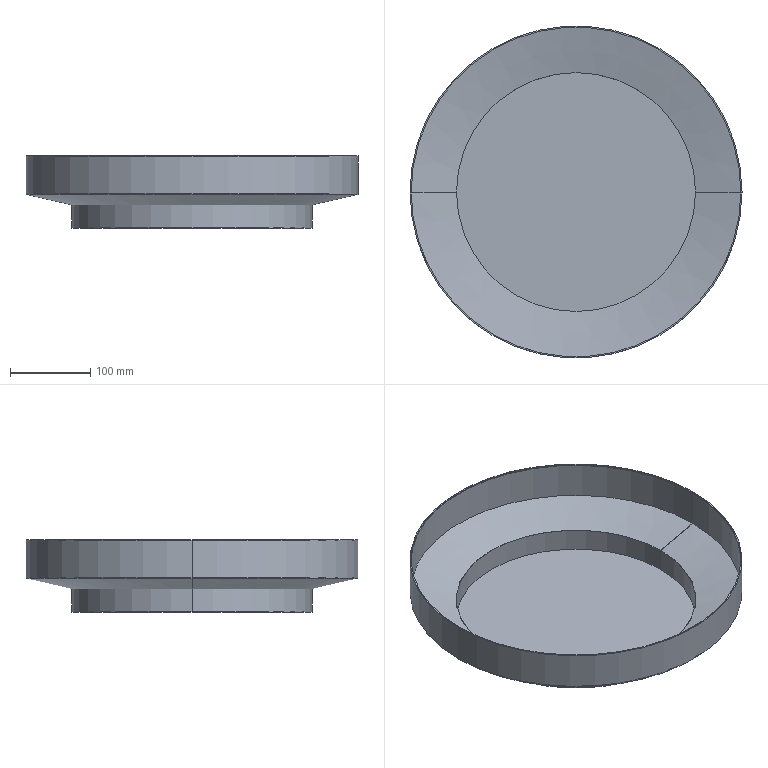Part | NX | 1 solid | 18 faces | box 414 x 414 x 90 mm | volume 225156 mm3 | cylinder 10 | plane 4 | cone 4 | commonest cylinder face diameters 298 x2 300 x2 411 x2 412 x2 414 x2
STEP:
#1=CARTESIAN_POINT('',(-186.483,-361.015,34.752));
#2=VERTEX_POINT('',#1);
#3=CARTESIAN_POINT('',(113.517,-361.015,34.752));
#4=VERTEX_POINT('',#3);
#5=CARTESIAN_POINT('',(-36.483,-361.015,34.752));
#6=DIRECTION('',(0.,0.,-1.));
#7=DIRECTION('',(1.,0.,0.));
#8=AXIS2_PLACEMENT_3D('',#5,#6,#7);
#9=CIRCLE('',#8,150.);
#10=EDGE_CURVE('',#2,#4,#9,.T.);
#11=ORIENTED_EDGE('',*,*,#10,.T.);
#12=CARTESIAN_POINT('',(-36.483,-361.015,34.752));
#13=DIRECTION('',(0.,0.,-1.));
#14=DIRECTION('',(1.,0.,0.));
#15=AXIS2_PLACEMENT_3D('',#12,#13,#14);
#16=CIRCLE('',#15,150.);
#17=EDGE_CURVE('',#4,#2,#16,.T.);
#18=ORIENTED_EDGE('',*,*,#17,.T.);
#19=EDGE_LOOP('',(#11,#18));
#20=FACE_BOUND('',#19,.T.);
#21=CARTESIAN_POINT('',(38.517,-361.015,34.752));
#22=DIRECTION('',(0.,0.,-1.));
#23=DIRECTION('',(0.,-1.,0.));
#24=AXIS2_PLACEMENT_3D('',#21,#22,#23);
#25=PLANE('',#24);
#26=ADVANCED_FACE('',(#20),#25,.T.);
#27=CARTESIAN_POINT('',(-186.483,-361.015,63.752));
#28=VERTEX_POINT('',#27);
#29=CARTESIAN_POINT('',(113.517,-361.015,63.752));
#30=VERTEX_POINT('',#29);
#31=CARTESIAN_POINT('',(-36.483,-361.015,63.752));
#32=DIRECTION('',(0.,0.,-1.));
#33=DIRECTION('',(1.,0.,0.));
#34=AXIS2_PLACEMENT_3D('',#31,#32,#33);
#35=CIRCLE('',#34,150.);
#36=EDGE_CURVE('',#28,#30,#35,.T.);
#37=ORIENTED_EDGE('',*,*,#36,.T.);
#38=CARTESIAN_POINT('',(113.517,-361.015,49.252));
#39=DIRECTION('',(0.,0.,1.));
#40=VECTOR('',#39,1000.);
#41=LINE('',#38,#40);
#42=EDGE_CURVE('',#4,#30,#41,.T.);
#43=ORIENTED_EDGE('',*,*,#42,.F.);
#44=ORIENTED_EDGE('',*,*,#10,.F.);
#45=CARTESIAN_POINT('',(-186.483,-361.015,49.252));
#46=DIRECTION('',(0.,0.,1.));
#47=VECTOR('',#46,1000.);
#48=LINE('',#45,#47);
#49=EDGE_CURVE('',#2,#28,#48,.T.);
#50=ORIENTED_EDGE('',*,*,#49,.T.);
#51=EDGE_LOOP('',(#37,#43,#44,#50));
#52=FACE_BOUND('',#51,.T.);
#53=CARTESIAN_POINT('',(-36.483,-361.015,49.252));
#54=DIRECTION('',(0.,0.,1.));
#55=DIRECTION('',(1.,0.,0.));
#56=AXIS2_PLACEMENT_3D('',#53,#54,#55);
#57=CYLINDRICAL_SURFACE('',#56,150.);
#58=ADVANCED_FACE('',(#52),#57,.T.);
#59=CARTESIAN_POINT('',(-243.483,-361.015,76.752));
#60=VERTEX_POINT('',#59);
#61=CARTESIAN_POINT('',(170.517,-361.015,76.752));
#62=VERTEX_POINT('',#61);
#63=CARTESIAN_POINT('',(-36.483,-361.015,76.752));
#64=DIRECTION('',(0.,0.,-1.));
#65=DIRECTION('',(1.,0.,0.));
#66=AXIS2_PLACEMENT_3D('',#63,#64,#65);
#67=CIRCLE('',#66,207.);
#68=EDGE_CURVE('',#60,#62,#67,.T.);
#69=ORIENTED_EDGE('',*,*,#68,.T.);
#70=CARTESIAN_POINT('',(170.517,-361.015,76.752));
#71=DIRECTION('',(0.975,0.,0.2224));
#72=VECTOR('',#71,1000.);
#73=LINE('',#70,#72);
#74=EDGE_CURVE('',#30,#62,#73,.T.);
#75=ORIENTED_EDGE('',*,*,#74,.F.);
#76=ORIENTED_EDGE('',*,*,#36,.F.);
#77=CARTESIAN_POINT('',(-243.483,-361.015,76.752));
#78=DIRECTION('',(-0.975,0.,0.2224));
#79=VECTOR('',#78,1000.);
#80=LINE('',#77,#79);
#81=EDGE_CURVE('',#28,#60,#80,.T.);
#82=ORIENTED_EDGE('',*,*,#81,.T.);
#83=EDGE_LOOP('',(#69,#75,#76,#82));
#84=FACE_BOUND('',#83,.T.);
#85=CARTESIAN_POINT('',(-36.483,-361.015,76.752));
#86=DIRECTION('',(0.,0.,1.));
#87=DIRECTION('',(1.,0.,0.));
#88=AXIS2_PLACEMENT_3D('',#85,#86,#87);
#89=CONICAL_SURFACE('',#88,207.,1.347);
#90=ADVANCED_FACE('',(#84),#89,.T.);
#91=CARTESIAN_POINT('',(-243.483,-361.015,124.752));
#92=VERTEX_POINT('',#91);
#93=CARTESIAN_POINT('',(170.517,-361.015,124.752));
#94=VERTEX_POINT('',#93);
#95=CARTESIAN_POINT('',(-36.483,-361.015,124.752));
#96=DIRECTION('',(0.,0.,-1.));
#97=DIRECTION('',(1.,0.,0.));
#98=AXIS2_PLACEMENT_3D('',#95,#96,#97);
#99=CIRCLE('',#98,207.);
#100=EDGE_CURVE('',#92,#94,#99,.T.);
#101=ORIENTED_EDGE('',*,*,#100,.T.);
#102=CARTESIAN_POINT('',(170.517,-361.015,100.752));
#103=DIRECTION('',(0.,0.,1.));
#104=VECTOR('',#103,1000.);
#105=LINE('',#102,#104);
#106=EDGE_CURVE('',#62,#94,#105,.T.);
#107=ORIENTED_EDGE('',*,*,#106,.F.);
#108=ORIENTED_EDGE('',*,*,#68,.F.);
#109=CARTESIAN_POINT('',(-243.483,-361.015,100.752));
#110=DIRECTION('',(0.,0.,1.));
#111=VECTOR('',#110,1000.);
#112=LINE('',#109,#111);
#113=EDGE_CURVE('',#60,#92,#112,.T.);
#114=ORIENTED_EDGE('',*,*,#113,.T.);
#115=EDGE_LOOP('',(#101,#107,#108,#114));
#116=FACE_BOUND('',#115,.T.);
#117=CARTESIAN_POINT('',(-36.483,-361.015,100.752));
#118=DIRECTION('',(0.,0.,1.));
#119=DIRECTION('',(1.,0.,0.));
#120=AXIS2_PLACEMENT_3D('',#117,#118,#119);
#121=CYLINDRICAL_SURFACE('',#120,207.);
#122=ADVANCED_FACE('',(#116),#121,.T.);
#123=ORIENTED_EDGE('',*,*,#100,.F.);
#124=CARTESIAN_POINT('',(-36.483,-361.015,124.752));
#125=DIRECTION('',(0.,0.,-1.));
#126=DIRECTION('',(1.,0.,0.));
#127=AXIS2_PLACEMENT_3D('',#124,#125,#126);
#128=CIRCLE('',#127,207.);
#129=EDGE_CURVE('',#94,#92,#128,.T.);
#130=ORIENTED_EDGE('',*,*,#129,.F.);
#131=EDGE_LOOP('',(#123,#130));
#132=FACE_BOUND('',#131,.T.);
#133=CARTESIAN_POINT('',(-241.983,-361.015,124.752));
#134=VERTEX_POINT('',#133);
#135=CARTESIAN_POINT('',(169.017,-361.015,124.752));
#136=VERTEX_POINT('',#135);
#137=CARTESIAN_POINT('',(-36.483,-361.015,124.752));
#138=DIRECTION('',(0.,0.,1.));
#139=DIRECTION('',(1.,0.,0.));
#140=AXIS2_PLACEMENT_3D('',#137,#138,#139);
#141=CIRCLE('',#140,205.5);
#142=EDGE_CURVE('',#134,#136,#141,.T.);
#143=ORIENTED_EDGE('',*,*,#142,.F.);
#144=CARTESIAN_POINT('',(-36.483,-361.015,124.752));
#145=DIRECTION('',(0.,0.,1.));
#146=DIRECTION('',(1.,0.,0.));
#147=AXIS2_PLACEMENT_3D('',#144,#145,#146);
#148=CIRCLE('',#147,205.5);
#149=EDGE_CURVE('',#136,#134,#148,.T.);
#150=ORIENTED_EDGE('',*,*,#149,.F.);
#151=EDGE_LOOP('',(#143,#150));
#152=FACE_BOUND('',#151,.T.);
#153=CARTESIAN_POINT('',(67.017,-361.015,124.752));
#154=DIRECTION('',(0.,0.,1.));
#155=DIRECTION('',(1.,0.,0.));
#156=AXIS2_PLACEMENT_3D('',#153,#154,#155);
#157=PLANE('',#156);
#158=ADVANCED_FACE('',(#132,#152),#157,.T.);
#159=CARTESIAN_POINT('',(-241.983,-361.015,123.752));
#160=VERTEX_POINT('',#159);
#161=CARTESIAN_POINT('',(169.017,-361.015,123.752));
#162=VERTEX_POINT('',#161);
#163=CARTESIAN_POINT('',(-36.483,-361.015,123.752));
#164=DIRECTION('',(0.,0.,1.));
#165=DIRECTION('',(1.,0.,0.));
#166=AXIS2_PLACEMENT_3D('',#163,#164,#165);
#167=CIRCLE('',#166,205.5);
#168=EDGE_CURVE('',#160,#162,#167,.T.);
#169=ORIENTED_EDGE('',*,*,#168,.F.);
#170=CARTESIAN_POINT('',(-241.983,-361.015,100.752));
#171=DIRECTION('',(0.,0.,1.));
#172=VECTOR('',#171,1000.);
#173=LINE('',#170,#172);
#174=EDGE_CURVE('',#160,#134,#173,.T.);
#175=ORIENTED_EDGE('',*,*,#174,.T.);
#176=ORIENTED_EDGE('',*,*,#142,.T.);
#177=CARTESIAN_POINT('',(169.017,-361.015,100.752));
#178=DIRECTION('',(0.,0.,1.));
#179=VECTOR('',#178,1000.);
#180=LINE('',#177,#179);
#181=EDGE_CURVE('',#162,#136,#180,.T.);
#182=ORIENTED_EDGE('',*,*,#181,.F.);
#183=EDGE_LOOP('',(#169,#175,#176,#182));
#184=FACE_BOUND('',#183,.T.);
#185=CARTESIAN_POINT('',(-36.483,-361.015,100.752));
#186=DIRECTION('',(0.,0.,1.));
#187=DIRECTION('',(1.,0.,0.));
#188=AXIS2_PLACEMENT_3D('',#185,#186,#187);
#189=CYLINDRICAL_SURFACE('',#188,205.5);
#190=ADVANCED_FACE('',(#184),#189,.F.);
#191=CARTESIAN_POINT('',(-242.483,-361.015,123.752));
#192=VERTEX_POINT('',#191);
#193=CARTESIAN_POINT('',(169.517,-361.015,123.752));
#194=VERTEX_POINT('',#193);
#195=CARTESIAN_POINT('',(-36.483,-361.015,123.752));
#196=DIRECTION('',(0.,0.,1.));
#197=DIRECTION('',(1.,0.,0.));
#198=AXIS2_PLACEMENT_3D('',#195,#196,#197);
#199=CIRCLE('',#198,206.);
#200=EDGE_CURVE('',#192,#194,#199,.T.);
#201=ORIENTED_EDGE('',*,*,#200,.F.);
#202=CARTESIAN_POINT('',(-36.483,-361.015,123.752));
#203=DIRECTION('',(0.,0.,1.));
#204=DIRECTION('',(1.,0.,0.));
#205=AXIS2_PLACEMENT_3D('',#202,#203,#204);
#206=CIRCLE('',#205,206.);
#207=EDGE_CURVE('',#194,#192,#206,.T.);
#208=ORIENTED_EDGE('',*,*,#207,.F.);
#209=EDGE_LOOP('',(#201,#208));
#210=FACE_BOUND('',#209,.T.);
#211=ORIENTED_EDGE('',*,*,#168,.T.);
#212=CARTESIAN_POINT('',(-36.483,-361.015,123.752));
#213=DIRECTION('',(0.,0.,1.));
#214=DIRECTION('',(1.,0.,0.));
#215=AXIS2_PLACEMENT_3D('',#212,#213,#214);
#216=CIRCLE('',#215,205.5);
#217=EDGE_CURVE('',#162,#160,#216,.T.);
#218=ORIENTED_EDGE('',*,*,#217,.T.);
#219=EDGE_LOOP('',(#211,#218));
#220=FACE_BOUND('',#219,.T.);
#221=CARTESIAN_POINT('',(67.017,-361.015,123.752));
#222=DIRECTION('',(0.,0.,1.));
#223=DIRECTION('',(1.,0.,0.));
#224=AXIS2_PLACEMENT_3D('',#221,#222,#223);
#225=PLANE('',#224);
#226=ADVANCED_FACE('',(#210,#220),#225,.F.);
#227=ORIENTED_EDGE('',*,*,#200,.T.);
#228=CARTESIAN_POINT('',(169.517,-361.015,77.549));
#229=VERTEX_POINT('',#228);
#230=CARTESIAN_POINT('',(169.517,-361.015,100.752));
#231=DIRECTION('',(0.,0.,1.));
#232=VECTOR('',#231,1000.);
#233=LINE('',#230,#232);
#234=EDGE_CURVE('',#229,#194,#233,.T.);
#235=ORIENTED_EDGE('',*,*,#234,.F.);
#236=CARTESIAN_POINT('',(-242.483,-361.015,77.549));
#237=VERTEX_POINT('',#236);
#238=CARTESIAN_POINT('',(-36.483,-361.015,77.549));
#239=DIRECTION('',(0.,0.,1.));
#240=DIRECTION('',(1.,0.,0.));
#241=AXIS2_PLACEMENT_3D('',#238,#239,#240);
#242=CIRCLE('',#241,206.);
#243=EDGE_CURVE('',#237,#229,#242,.T.);
#244=ORIENTED_EDGE('',*,*,#243,.F.);
#245=CARTESIAN_POINT('',(-242.483,-361.015,100.752));
#246=DIRECTION('',(0.,0.,1.));
#247=VECTOR('',#246,1000.);
#248=LINE('',#245,#247);
#249=EDGE_CURVE('',#237,#192,#248,.T.);
#250=ORIENTED_EDGE('',*,*,#249,.T.);
#251=EDGE_LOOP('',(#227,#235,#244,#250));
#252=FACE_BOUND('',#251,.T.);
#253=CARTESIAN_POINT('',(-36.483,-361.015,100.752));
#254=DIRECTION('',(0.,0.,1.));
#255=DIRECTION('',(1.,0.,0.));
#256=AXIS2_PLACEMENT_3D('',#253,#254,#255);
#257=CYLINDRICAL_SURFACE('',#256,206.);
#258=ADVANCED_FACE('',(#252),#257,.F.);
#259=ORIENTED_EDGE('',*,*,#243,.T.);
#260=CARTESIAN_POINT('',(112.517,-361.015,64.549));
#261=VERTEX_POINT('',#260);
#262=CARTESIAN_POINT('',(170.517,-361.015,77.777));
#263=DIRECTION('',(0.975,0.,0.2224));
#264=VECTOR('',#263,1000.);
#265=LINE('',#262,#264);
#266=EDGE_CURVE('',#261,#229,#265,.T.);
#267=ORIENTED_EDGE('',*,*,#266,.F.);
#268=CARTESIAN_POINT('',(-185.483,-361.015,64.549));
#269=VERTEX_POINT('',#268);
#270=CARTESIAN_POINT('',(-36.483,-361.015,64.549));
#271=DIRECTION('',(0.,0.,1.));
#272=DIRECTION('',(1.,0.,0.));
#273=AXIS2_PLACEMENT_3D('',#270,#271,#272);
#274=CIRCLE('',#273,149.);
#275=EDGE_CURVE('',#269,#261,#274,.T.);
#276=ORIENTED_EDGE('',*,*,#275,.F.);
#277=CARTESIAN_POINT('',(-243.483,-361.015,77.777));
#278=DIRECTION('',(-0.975,0.,0.2224));
#279=VECTOR('',#278,1000.);
#280=LINE('',#277,#279);
#281=EDGE_CURVE('',#269,#237,#280,.T.);
#282=ORIENTED_EDGE('',*,*,#281,.T.);
#283=EDGE_LOOP('',(#259,#267,#276,#282));
#284=FACE_BOUND('',#283,.T.);
#285=CARTESIAN_POINT('',(-36.483,-361.015,77.777));
#286=DIRECTION('',(0.,0.,1.));
#287=DIRECTION('',(1.,0.,0.));
#288=AXIS2_PLACEMENT_3D('',#285,#286,#287);
#289=CONICAL_SURFACE('',#288,207.,1.347);
#290=ADVANCED_FACE('',(#284),#289,.F.);
#291=ORIENTED_EDGE('',*,*,#275,.T.);
#292=CARTESIAN_POINT('',(112.517,-361.015,35.752));
#293=VERTEX_POINT('',#292);
#294=CARTESIAN_POINT('',(112.517,-361.015,49.252));
#295=DIRECTION('',(0.,0.,1.));
#296=VECTOR('',#295,1000.);
#297=LINE('',#294,#296);
#298=EDGE_CURVE('',#293,#261,#297,.T.);
#299=ORIENTED_EDGE('',*,*,#298,.F.);
#300=CARTESIAN_POINT('',(-185.483,-361.015,35.752));
#301=VERTEX_POINT('',#300);
#302=CARTESIAN_POINT('',(-36.483,-361.015,35.752));
#303=DIRECTION('',(0.,0.,1.));
#304=DIRECTION('',(1.,0.,0.));
#305=AXIS2_PLACEMENT_3D('',#302,#303,#304);
#306=CIRCLE('',#305,149.);
#307=EDGE_CURVE('',#301,#293,#306,.T.);
#308=ORIENTED_EDGE('',*,*,#307,.F.);
#309=CARTESIAN_POINT('',(-185.483,-361.015,49.252));
#310=DIRECTION('',(0.,0.,1.));
#311=VECTOR('',#310,1000.);
#312=LINE('',#309,#311);
#313=EDGE_CURVE('',#301,#269,#312,.T.);
#314=ORIENTED_EDGE('',*,*,#313,.T.);
#315=EDGE_LOOP('',(#291,#299,#308,#314));
#316=FACE_BOUND('',#315,.T.);
#317=CARTESIAN_POINT('',(-36.483,-361.015,49.252));
#318=DIRECTION('',(0.,0.,1.));
#319=DIRECTION('',(1.,0.,0.));
#320=AXIS2_PLACEMENT_3D('',#317,#318,#319);
#321=CYLINDRICAL_SURFACE('',#320,149.);
#322=ADVANCED_FACE('',(#316),#321,.F.);
#323=ORIENTED_EDGE('',*,*,#307,.T.);
#324=CARTESIAN_POINT('',(-36.483,-361.015,35.752));
#325=DIRECTION('',(0.,0.,1.));
#326=DIRECTION('',(1.,0.,0.));
#327=AXIS2_PLACEMENT_3D('',#324,#325,#326);
#328=CIRCLE('',#327,149.);
#329=EDGE_CURVE('',#293,#301,#328,.T.);
#330=ORIENTED_EDGE('',*,*,#329,.T.);
#331=EDGE_LOOP('',(#323,#330));
#332=FACE_BOUND('',#331,.T.);
#333=CARTESIAN_POINT('',(38.517,-361.015,35.752));
#334=DIRECTION('',(0.,0.,-1.));
#335=DIRECTION('',(0.,-1.,0.));
#336=AXIS2_PLACEMENT_3D('',#333,#334,#335);
#337=PLANE('',#336);
#338=ADVANCED_FACE('',(#332),#337,.F.);
#339=ORIENTED_EDGE('',*,*,#234,.T.);
#340=ORIENTED_EDGE('',*,*,#207,.T.);
#341=ORIENTED_EDGE('',*,*,#249,.F.);
#342=CARTESIAN_POINT('',(-36.483,-361.015,77.549));
#343=DIRECTION('',(0.,0.,1.));
#344=DIRECTION('',(1.,0.,0.));
#345=AXIS2_PLACEMENT_3D('',#342,#343,#344);
#346=CIRCLE('',#345,206.);
#347=EDGE_CURVE('',#229,#237,#346,.T.);
#348=ORIENTED_EDGE('',*,*,#347,.F.);
#349=EDGE_LOOP('',(#339,#340,#341,#348));
#350=FACE_BOUND('',#349,.T.);
#351=CARTESIAN_POINT('',(-36.483,-361.015,100.752));
#352=DIRECTION('',(0.,0.,1.));
#353=DIRECTION('',(1.,0.,0.));
#354=AXIS2_PLACEMENT_3D('',#351,#352,#353);
#355=CYLINDRICAL_SURFACE('',#354,206.);
#356=ADVANCED_FACE('',(#350),#355,.F.);
#357=ORIENTED_EDGE('',*,*,#181,.T.);
#358=ORIENTED_EDGE('',*,*,#149,.T.);
#359=ORIENTED_EDGE('',*,*,#174,.F.);
#360=ORIENTED_EDGE('',*,*,#217,.F.);
#361=EDGE_LOOP('',(#357,#358,#359,#360));
#362=FACE_BOUND('',#361,.T.);
#363=CARTESIAN_POINT('',(-36.483,-361.015,100.752));
#364=DIRECTION('',(0.,0.,1.));
#365=DIRECTION('',(1.,0.,0.));
#366=AXIS2_PLACEMENT_3D('',#363,#364,#365);
#367=CYLINDRICAL_SURFACE('',#366,205.5);
#368=ADVANCED_FACE('',(#362),#367,.F.);
#369=ORIENTED_EDGE('',*,*,#106,.T.);
#370=ORIENTED_EDGE('',*,*,#129,.T.);
#371=ORIENTED_EDGE('',*,*,#113,.F.);
#372=CARTESIAN_POINT('',(-36.483,-361.015,76.752));
#373=DIRECTION('',(0.,0.,-1.));
#374=DIRECTION('',(1.,0.,0.));
#375=AXIS2_PLACEMENT_3D('',#372,#373,#374);
#376=CIRCLE('',#375,207.);
#377=EDGE_CURVE('',#62,#60,#376,.T.);
#378=ORIENTED_EDGE('',*,*,#377,.F.);
#379=EDGE_LOOP('',(#369,#370,#371,#378));
#380=FACE_BOUND('',#379,.T.);
#381=CARTESIAN_POINT('',(-36.483,-361.015,100.752));
#382=DIRECTION('',(0.,0.,1.));
#383=DIRECTION('',(1.,0.,0.));
#384=AXIS2_PLACEMENT_3D('',#381,#382,#383);
#385=CYLINDRICAL_SURFACE('',#384,207.);
#386=ADVANCED_FACE('',(#380),#385,.T.);
#387=ORIENTED_EDGE('',*,*,#298,.T.);
#388=CARTESIAN_POINT('',(-36.483,-361.015,64.549));
#389=DIRECTION('',(0.,0.,1.));
#390=DIRECTION('',(1.,0.,0.));
#391=AXIS2_PLACEMENT_3D('',#388,#389,#390);
#392=CIRCLE('',#391,149.);
#393=EDGE_CURVE('',#261,#269,#392,.T.);
#394=ORIENTED_EDGE('',*,*,#393,.T.);
#395=ORIENTED_EDGE('',*,*,#313,.F.);
#396=ORIENTED_EDGE('',*,*,#329,.F.);
#397=EDGE_LOOP('',(#387,#394,#395,#396));
#398=FACE_BOUND('',#397,.T.);
#399=CARTESIAN_POINT('',(-36.483,-361.015,49.252));
#400=DIRECTION('',(0.,0.,1.));
#401=DIRECTION('',(1.,0.,0.));
#402=AXIS2_PLACEMENT_3D('',#399,#400,#401);
#403=CYLINDRICAL_SURFACE('',#402,149.);
#404=ADVANCED_FACE('',(#398),#403,.F.);
#405=ORIENTED_EDGE('',*,*,#74,.T.);
#406=ORIENTED_EDGE('',*,*,#377,.T.);
#407=ORIENTED_EDGE('',*,*,#81,.F.);
#408=CARTESIAN_POINT('',(-36.483,-361.015,63.752));
#409=DIRECTION('',(0.,0.,-1.));
#410=DIRECTION('',(1.,0.,0.));
#411=AXIS2_PLACEMENT_3D('',#408,#409,#410);
#412=CIRCLE('',#411,150.);
#413=EDGE_CURVE('',#30,#28,#412,.T.);
#414=ORIENTED_EDGE('',*,*,#413,.F.);
#415=EDGE_LOOP('',(#405,#406,#407,#414));
#416=FACE_BOUND('',#415,.T.);
#417=CARTESIAN_POINT('',(-36.483,-361.015,76.752));
#418=DIRECTION('',(0.,0.,1.));
#419=DIRECTION('',(1.,0.,0.));
#420=AXIS2_PLACEMENT_3D('',#417,#418,#419);
#421=CONICAL_SURFACE('',#420,207.,1.347);
#422=ADVANCED_FACE('',(#416),#421,.T.);
#423=ORIENTED_EDGE('',*,*,#266,.T.);
#424=ORIENTED_EDGE('',*,*,#347,.T.);
#425=ORIENTED_EDGE('',*,*,#281,.F.);
#426=ORIENTED_EDGE('',*,*,#393,.F.);
#427=EDGE_LOOP('',(#423,#424,#425,#426));
#428=FACE_BOUND('',#427,.T.);
#429=CARTESIAN_POINT('',(-36.483,-361.015,77.777));
#430=DIRECTION('',(0.,0.,1.));
#431=DIRECTION('',(1.,0.,0.));
#432=AXIS2_PLACEMENT_3D('',#429,#430,#431);
#433=CONICAL_SURFACE('',#432,207.,1.347);
#434=ADVANCED_FACE('',(#428),#433,.F.);
#435=ORIENTED_EDGE('',*,*,#42,.T.);
#436=ORIENTED_EDGE('',*,*,#413,.T.);
#437=ORIENTED_EDGE('',*,*,#49,.F.);
#438=ORIENTED_EDGE('',*,*,#17,.F.);
#439=EDGE_LOOP('',(#435,#436,#437,#438));
#440=FACE_BOUND('',#439,.T.);
#441=CARTESIAN_POINT('',(-36.483,-361.015,49.252));
#442=DIRECTION('',(0.,0.,1.));
#443=DIRECTION('',(1.,0.,0.));
#444=AXIS2_PLACEMENT_3D('',#441,#442,#443);
#445=CYLINDRICAL_SURFACE('',#444,150.);
#446=ADVANCED_FACE('',(#440),#445,.T.);
#447=CLOSED_SHELL('',(#26,#58,#90,#122,#158,#190,#226,#258,#290,#322,#338,#356,#368,#386,#404,#422,#434,#446));
#448=MANIFOLD_SOLID_BREP('',#447);
#449=(LENGTH_UNIT()NAMED_UNIT(*)SI_UNIT(.MILLI.,.METRE.));
#450=UNCERTAINTY_MEASURE_WITH_UNIT(LENGTH_MEASURE(0.00001),#449,'','');
#451=(NAMED_UNIT(*)PLANE_ANGLE_UNIT()SI_UNIT($,.RADIAN.));
#452=(NAMED_UNIT(*)SI_UNIT($,.STERADIAN.)SOLID_ANGLE_UNIT());
#453=(GEOMETRIC_REPRESENTATION_CONTEXT(3)GLOBAL_UNCERTAINTY_ASSIGNED_CONTEXT((#450))GLOBAL_UNIT_ASSIGNED_CONTEXT((#449,#451,#452))REPRESENTATION_CONTEXT('',''));
#454=ADVANCED_BREP_SHAPE_REPRESENTATION('',(#448),#453);